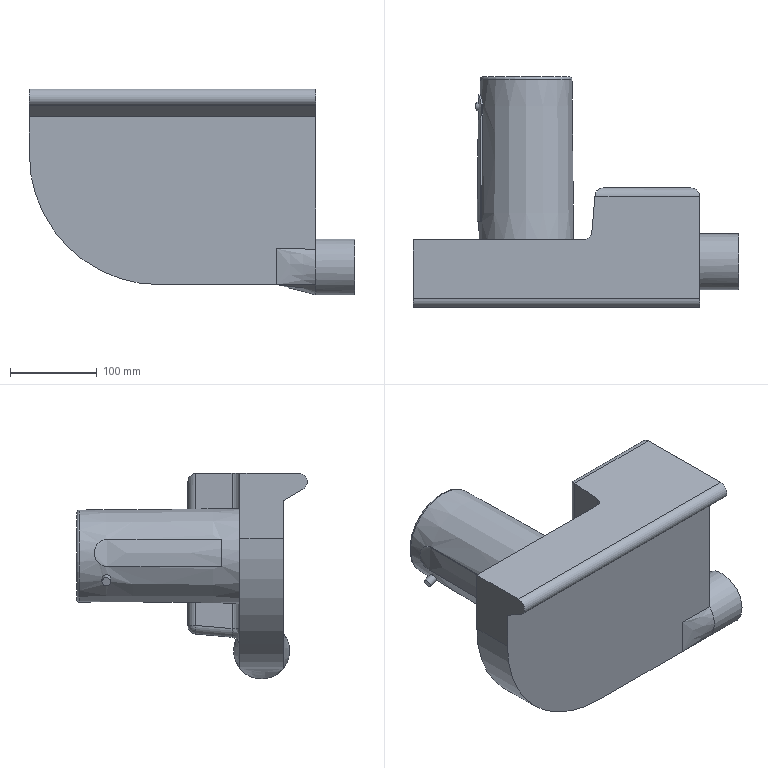Part | STEP file | DEWALT-DWE7492-B2_23 | 1 solid | 40 faces | box 375 x 265.806 x 237.3 mm | volume 6943918 mm3 | plane 15 | cylinder 11 | spline 10 | cone 2 | torus 1 | sphere 1 | commonest cylinder face diameters 20 x8 10 x1 64.6 x1 300 x1